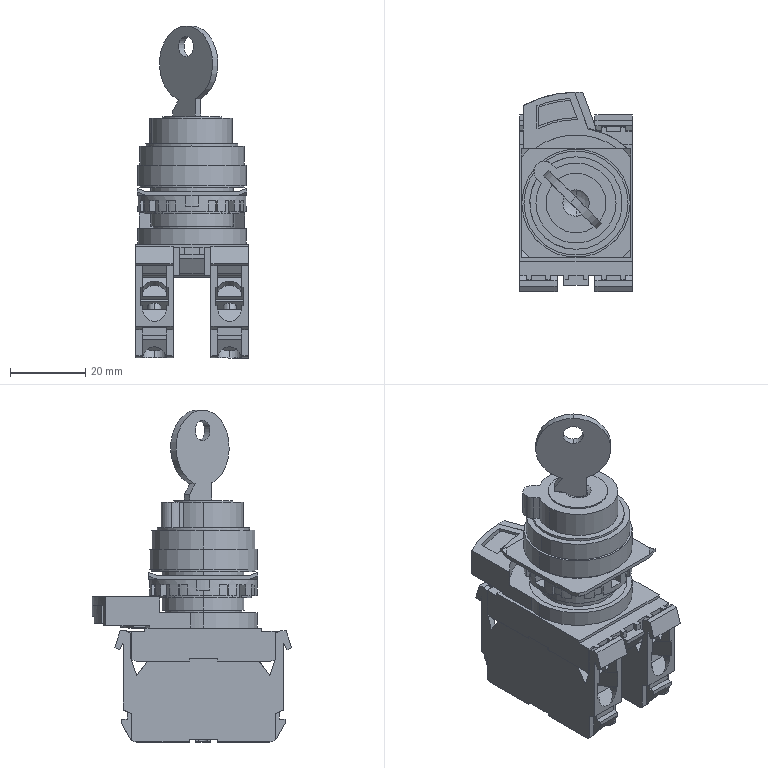Part | STEP file | A22NK_2BM_01AA_G102 | 7 solids | 731 faces | box 30 x 53 x 88.3 mm | volume 39098 mm3 | plane 584 | cylinder 144 | sphere 3 | commonest cylinder face diameters 6.5 x12 4 x10 25.4 x10 3.5 x8 5.8 x8 6 x8